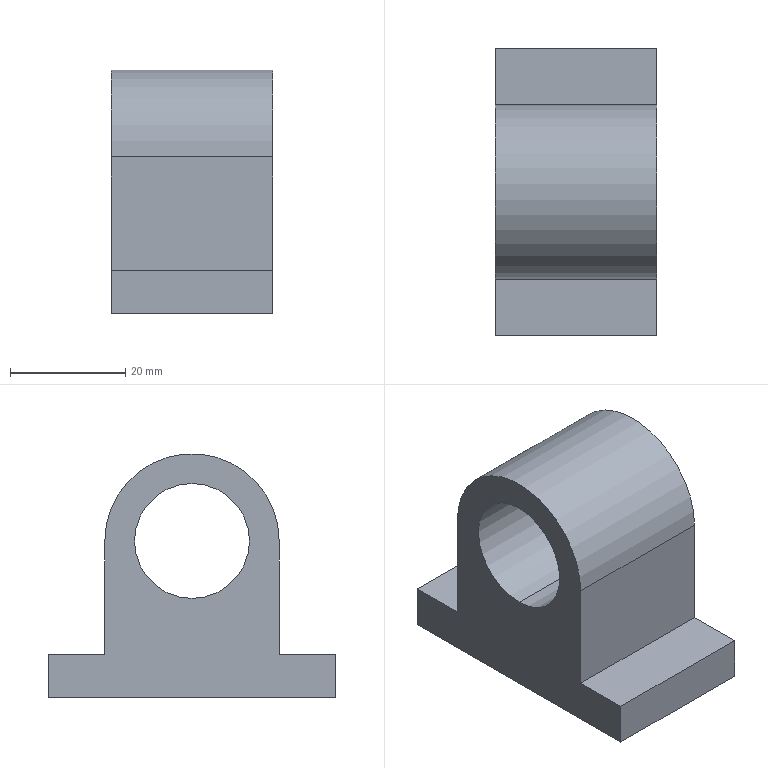Part | STEP file | 1 solid | 12 faces | box 28 x 50 x 42.426 mm | volume 28637 mm3 | plane 9 | cylinder 3 | commonest cylinder face diameters 20 x2 30.309 x1
STEP:
#1=CARTESIAN_POINT('',(0.,0.,0.));
#2=DIRECTION('',(0.,0.,1.));
#3=DIRECTION('',(1.,0.,0.));
#4=AXIS2_PLACEMENT_3D('',#1,#2,#3);
#5=CARTESIAN_POINT('',(572.,553.5,94.906));
#6=VERTEX_POINT('',#5);
#7=CARTESIAN_POINT('',(600.,553.5,94.906));
#8=VERTEX_POINT('',#7);
#9=CARTESIAN_POINT('',(572.,553.5,94.906));
#10=DIRECTION('',(1.,0.,0.));
#11=VECTOR('',#10,1.);
#12=LINE('',#9,#11);
#13=CARTESIAN_POINT('',(572.,553.5,104.906));
#14=DIRECTION('',(1.,0.,0.));
#15=DIRECTION('',(0.,0.,-1.));
#16=AXIS2_PLACEMENT_3D('',#13,#14,#15);
#17=CYLINDRICAL_SURFACE('',#16,10.);
#18=CARTESIAN_POINT('',(6.283,0.));
#19=DIRECTION('',(0.,1.));
#20=VECTOR('',#19,1.);
#21=LINE('',#18,#20);
#22=(GEOMETRIC_REPRESENTATION_CONTEXT(2)PARAMETRIC_REPRESENTATION_CONTEXT()REPRESENTATION_CONTEXT('',''));
#23=DEFINITIONAL_REPRESENTATION('',(#21),#22);
#24=PCURVE('',#17,#23);
#25=CARTESIAN_POINT('',(572.,553.5,104.906));
#26=DIRECTION('',(1.,0.,0.));
#27=DIRECTION('',(0.,0.,-1.));
#28=AXIS2_PLACEMENT_3D('',#25,#26,#27);
#29=CYLINDRICAL_SURFACE('',#28,10.);
#30=CARTESIAN_POINT('',(0.,0.));
#31=DIRECTION('',(0.,1.));
#32=VECTOR('',#31,1.);
#33=LINE('',#30,#32);
#34=(GEOMETRIC_REPRESENTATION_CONTEXT(2)PARAMETRIC_REPRESENTATION_CONTEXT()REPRESENTATION_CONTEXT('',''));
#35=DEFINITIONAL_REPRESENTATION('',(#33),#34);
#36=PCURVE('',#29,#35);
#37=SURFACE_CURVE('',#12,(#24,#36),.PCURVE_S1.);
#38=EDGE_CURVE('',#6,#8,#37,.T.);
#39=ORIENTED_EDGE('',*,*,#38,.T.);
#40=CARTESIAN_POINT('',(600.,553.5,114.906));
#41=VERTEX_POINT('',#40);
#42=CARTESIAN_POINT('',(600.,553.5,104.906));
#43=DIRECTION('',(1.,0.,0.));
#44=DIRECTION('',(0.,0.,-1.));
#45=AXIS2_PLACEMENT_3D('',#42,#43,#44);
#46=CIRCLE('',#45,10.);
#47=CARTESIAN_POINT('',(0.,28.));
#48=DIRECTION('',(1.,0.));
#49=VECTOR('',#48,1.);
#50=LINE('',#47,#49);
#51=(GEOMETRIC_REPRESENTATION_CONTEXT(2)PARAMETRIC_REPRESENTATION_CONTEXT()REPRESENTATION_CONTEXT('',''));
#52=DEFINITIONAL_REPRESENTATION('',(#50),#51);
#53=PCURVE('',#17,#52);
#54=CARTESIAN_POINT('',(600.,553.5,104.906));
#55=DIRECTION('',(1.,0.,0.));
#56=DIRECTION('',(0.,0.,-1.));
#57=AXIS2_PLACEMENT_3D('',#54,#55,#56);
#58=PLANE('',#57);
#59=CARTESIAN_POINT('',(0.,0.));
#60=DIRECTION('',(1.,0.));
#61=AXIS2_PLACEMENT_2D('',#59,#60);
#62=CIRCLE('',#61,10.);
#63=(GEOMETRIC_REPRESENTATION_CONTEXT(2)PARAMETRIC_REPRESENTATION_CONTEXT()REPRESENTATION_CONTEXT('',''));
#64=DEFINITIONAL_REPRESENTATION('',(#62),#63);
#65=PCURVE('',#58,#64);
#66=SURFACE_CURVE('',#46,(#53,#65),.PCURVE_S1.);
#67=EDGE_CURVE('',#41,#8,#66,.T.);
#68=ORIENTED_EDGE('',*,*,#67,.F.);
#69=CARTESIAN_POINT('',(572.,553.5,114.906));
#70=VERTEX_POINT('',#69);
#71=CARTESIAN_POINT('',(572.,553.5,114.906));
#72=DIRECTION('',(1.,0.,0.));
#73=VECTOR('',#72,1.);
#74=LINE('',#71,#73);
#75=CARTESIAN_POINT('',(3.142,0.));
#76=DIRECTION('',(0.,1.));
#77=VECTOR('',#76,1.);
#78=LINE('',#75,#77);
#79=(GEOMETRIC_REPRESENTATION_CONTEXT(2)PARAMETRIC_REPRESENTATION_CONTEXT()REPRESENTATION_CONTEXT('',''));
#80=DEFINITIONAL_REPRESENTATION('',(#78),#79);
#81=PCURVE('',#17,#80);
#82=CARTESIAN_POINT('',(3.142,0.));
#83=DIRECTION('',(0.,1.));
#84=VECTOR('',#83,1.);
#85=LINE('',#82,#84);
#86=(GEOMETRIC_REPRESENTATION_CONTEXT(2)PARAMETRIC_REPRESENTATION_CONTEXT()REPRESENTATION_CONTEXT('',''));
#87=DEFINITIONAL_REPRESENTATION('',(#85),#86);
#88=PCURVE('',#29,#87);
#89=SURFACE_CURVE('',#74,(#81,#88),.PCURVE_S1.);
#90=EDGE_CURVE('',#70,#41,#89,.T.);
#91=ORIENTED_EDGE('',*,*,#90,.F.);
#92=CARTESIAN_POINT('',(572.,553.5,104.906));
#93=DIRECTION('',(1.,0.,0.));
#94=DIRECTION('',(0.,0.,-1.));
#95=AXIS2_PLACEMENT_3D('',#92,#93,#94);
#96=CIRCLE('',#95,10.);
#97=CARTESIAN_POINT('',(0.,0.));
#98=DIRECTION('',(1.,0.));
#99=VECTOR('',#98,1.);
#100=LINE('',#97,#99);
#101=(GEOMETRIC_REPRESENTATION_CONTEXT(2)PARAMETRIC_REPRESENTATION_CONTEXT()REPRESENTATION_CONTEXT('',''));
#102=DEFINITIONAL_REPRESENTATION('',(#100),#101);
#103=PCURVE('',#17,#102);
#104=CARTESIAN_POINT('',(572.,553.5,104.906));
#105=DIRECTION('',(1.,0.,0.));
#106=DIRECTION('',(0.,0.,-1.));
#107=AXIS2_PLACEMENT_3D('',#104,#105,#106);
#108=PLANE('',#107);
#109=CARTESIAN_POINT('',(0.,0.));
#110=DIRECTION('',(1.,0.));
#111=AXIS2_PLACEMENT_2D('',#109,#110);
#112=CIRCLE('',#111,10.);
#113=(GEOMETRIC_REPRESENTATION_CONTEXT(2)PARAMETRIC_REPRESENTATION_CONTEXT()REPRESENTATION_CONTEXT('',''));
#114=DEFINITIONAL_REPRESENTATION('',(#112),#113);
#115=PCURVE('',#108,#114);
#116=SURFACE_CURVE('',#96,(#103,#115),.PCURVE_S1.);
#117=EDGE_CURVE('',#70,#6,#116,.T.);
#118=ORIENTED_EDGE('',*,*,#117,.T.);
#119=EDGE_LOOP('',(#39,#68,#91,#118));
#120=FACE_BOUND('',#119,.F.);
#121=ADVANCED_FACE('',(#120),#17,.F.);
#122=CARTESIAN_POINT('',(600.,528.5,77.635));
#123=VERTEX_POINT('',#122);
#124=CARTESIAN_POINT('',(600.,578.5,77.635));
#125=VERTEX_POINT('',#124);
#126=CARTESIAN_POINT('',(600.,578.5,77.635));
#127=DIRECTION('',(0.,1.,0.));
#128=VECTOR('',#127,1.);
#129=LINE('',#126,#128);
#130=CARTESIAN_POINT('',(572.,578.5,77.635));
#131=DIRECTION('',(0.,0.,-1.));
#132=DIRECTION('',(-1.,0.,0.));
#133=AXIS2_PLACEMENT_3D('',#130,#131,#132);
#134=PLANE('',#133);
#135=CARTESIAN_POINT('',(-28.,0.));
#136=DIRECTION('',(0.,1.));
#137=VECTOR('',#136,1.);
#138=LINE('',#135,#137);
#139=(GEOMETRIC_REPRESENTATION_CONTEXT(2)PARAMETRIC_REPRESENTATION_CONTEXT()REPRESENTATION_CONTEXT('',''));
#140=DEFINITIONAL_REPRESENTATION('',(#138),#139);
#141=PCURVE('',#134,#140);
#142=CARTESIAN_POINT('',(27.271,25.));
#143=DIRECTION('',(0.,1.));
#144=VECTOR('',#143,1.);
#145=LINE('',#142,#144);
#146=(GEOMETRIC_REPRESENTATION_CONTEXT(2)PARAMETRIC_REPRESENTATION_CONTEXT()REPRESENTATION_CONTEXT('',''));
#147=DEFINITIONAL_REPRESENTATION('',(#145),#146);
#148=PCURVE('',#58,#147);
#149=SURFACE_CURVE('',#129,(#141,#148),.PCURVE_S1.);
#150=EDGE_CURVE('',#123,#125,#149,.T.);
#151=ORIENTED_EDGE('',*,*,#150,.F.);
#152=CARTESIAN_POINT('',(572.,528.5,77.635));
#153=VERTEX_POINT('',#152);
#154=CARTESIAN_POINT('',(572.,528.5,77.635));
#155=DIRECTION('',(1.,0.,0.));
#156=VECTOR('',#155,1.);
#157=LINE('',#154,#156);
#158=CARTESIAN_POINT('',(0.,-50.));
#159=DIRECTION('',(-1.,0.));
#160=VECTOR('',#159,1.);
#161=LINE('',#158,#160);
#162=(GEOMETRIC_REPRESENTATION_CONTEXT(2)PARAMETRIC_REPRESENTATION_CONTEXT()REPRESENTATION_CONTEXT('',''));
#163=DEFINITIONAL_REPRESENTATION('',(#161),#162);
#164=PCURVE('',#134,#163);
#165=CARTESIAN_POINT('',(572.,528.5,77.635));
#166=DIRECTION('',(0.,-1.,0.));
#167=DIRECTION('',(0.,0.,-1.));
#168=AXIS2_PLACEMENT_3D('',#165,#166,#167);
#169=PLANE('',#168);
#170=CARTESIAN_POINT('',(0.,0.));
#171=DIRECTION('',(0.,1.));
#172=VECTOR('',#171,1.);
#173=LINE('',#170,#172);
#174=(GEOMETRIC_REPRESENTATION_CONTEXT(2)PARAMETRIC_REPRESENTATION_CONTEXT()REPRESENTATION_CONTEXT('',''));
#175=DEFINITIONAL_REPRESENTATION('',(#173),#174);
#176=PCURVE('',#169,#175);
#177=SURFACE_CURVE('',#157,(#164,#176),.PCURVE_S1.);
#178=EDGE_CURVE('',#153,#123,#177,.T.);
#179=ORIENTED_EDGE('',*,*,#178,.F.);
#180=CARTESIAN_POINT('',(572.,578.5,77.635));
#181=VERTEX_POINT('',#180);
#182=CARTESIAN_POINT('',(572.,578.5,77.635));
#183=DIRECTION('',(0.,1.,0.));
#184=VECTOR('',#183,1.);
#185=LINE('',#182,#184);
#186=CARTESIAN_POINT('',(0.,0.));
#187=DIRECTION('',(0.,1.));
#188=VECTOR('',#187,1.);
#189=LINE('',#186,#188);
#190=(GEOMETRIC_REPRESENTATION_CONTEXT(2)PARAMETRIC_REPRESENTATION_CONTEXT()REPRESENTATION_CONTEXT('',''));
#191=DEFINITIONAL_REPRESENTATION('',(#189),#190);
#192=PCURVE('',#134,#191);
#193=CARTESIAN_POINT('',(27.271,25.));
#194=DIRECTION('',(0.,1.));
#195=VECTOR('',#194,1.);
#196=LINE('',#193,#195);
#197=(GEOMETRIC_REPRESENTATION_CONTEXT(2)PARAMETRIC_REPRESENTATION_CONTEXT()REPRESENTATION_CONTEXT('',''));
#198=DEFINITIONAL_REPRESENTATION('',(#196),#197);
#199=PCURVE('',#108,#198);
#200=SURFACE_CURVE('',#185,(#192,#199),.PCURVE_S1.);
#201=EDGE_CURVE('',#153,#181,#200,.T.);
#202=ORIENTED_EDGE('',*,*,#201,.T.);
#203=CARTESIAN_POINT('',(572.,578.5,77.635));
#204=DIRECTION('',(1.,0.,0.));
#205=VECTOR('',#204,1.);
#206=LINE('',#203,#205);
#207=CARTESIAN_POINT('',(0.,0.));
#208=DIRECTION('',(-1.,0.));
#209=VECTOR('',#208,1.);
#210=LINE('',#207,#209);
#211=(GEOMETRIC_REPRESENTATION_CONTEXT(2)PARAMETRIC_REPRESENTATION_CONTEXT()REPRESENTATION_CONTEXT('',''));
#212=DEFINITIONAL_REPRESENTATION('',(#210),#211);
#213=PCURVE('',#134,#212);
#214=CARTESIAN_POINT('',(572.,578.5,77.635));
#215=DIRECTION('',(0.,1.,0.));
#216=DIRECTION('',(0.,0.,1.));
#217=AXIS2_PLACEMENT_3D('',#214,#215,#216);
#218=PLANE('',#217);
#219=CARTESIAN_POINT('',(0.,0.));
#220=DIRECTION('',(0.,1.));
#221=VECTOR('',#220,1.);
#222=LINE('',#219,#221);
#223=(GEOMETRIC_REPRESENTATION_CONTEXT(2)PARAMETRIC_REPRESENTATION_CONTEXT()REPRESENTATION_CONTEXT('',''));
#224=DEFINITIONAL_REPRESENTATION('',(#222),#223);
#225=PCURVE('',#218,#224);
#226=SURFACE_CURVE('',#206,(#213,#225),.PCURVE_S1.);
#227=EDGE_CURVE('',#181,#125,#226,.T.);
#228=ORIENTED_EDGE('',*,*,#227,.T.);
#229=EDGE_LOOP('',(#151,#179,#202,#228));
#230=FACE_BOUND('',#229,.T.);
#231=ADVANCED_FACE('',(#230),#134,.T.);
#232=CARTESIAN_POINT('',(600.,528.5,85.232));
#233=VERTEX_POINT('',#232);
#234=CARTESIAN_POINT('',(600.,528.5,77.635));
#235=DIRECTION('',(0.,0.,-1.));
#236=VECTOR('',#235,1.);
#237=LINE('',#234,#236);
#238=CARTESIAN_POINT('',(0.,28.));
#239=DIRECTION('',(1.,0.));
#240=VECTOR('',#239,1.);
#241=LINE('',#238,#240);
#242=(GEOMETRIC_REPRESENTATION_CONTEXT(2)PARAMETRIC_REPRESENTATION_CONTEXT()REPRESENTATION_CONTEXT('',''));
#243=DEFINITIONAL_REPRESENTATION('',(#241),#242);
#244=PCURVE('',#169,#243);
#245=CARTESIAN_POINT('',(27.271,-25.));
#246=DIRECTION('',(1.,0.));
#247=VECTOR('',#246,1.);
#248=LINE('',#245,#247);
#249=(GEOMETRIC_REPRESENTATION_CONTEXT(2)PARAMETRIC_REPRESENTATION_CONTEXT()REPRESENTATION_CONTEXT('',''));
#250=DEFINITIONAL_REPRESENTATION('',(#248),#249);
#251=PCURVE('',#58,#250);
#252=SURFACE_CURVE('',#237,(#244,#251),.PCURVE_S1.);
#253=EDGE_CURVE('',#233,#123,#252,.T.);
#254=ORIENTED_EDGE('',*,*,#253,.F.);
#255=CARTESIAN_POINT('',(572.,528.5,85.232));
#256=VERTEX_POINT('',#255);
#257=CARTESIAN_POINT('',(572.,528.5,85.232));
#258=DIRECTION('',(1.,0.,0.));
#259=VECTOR('',#258,1.);
#260=LINE('',#257,#259);
#261=CARTESIAN_POINT('',(-7.597,0.));
#262=DIRECTION('',(0.,1.));
#263=VECTOR('',#262,1.);
#264=LINE('',#261,#263);
#265=(GEOMETRIC_REPRESENTATION_CONTEXT(2)PARAMETRIC_REPRESENTATION_CONTEXT()REPRESENTATION_CONTEXT('',''));
#266=DEFINITIONAL_REPRESENTATION('',(#264),#265);
#267=PCURVE('',#169,#266);
#268=CARTESIAN_POINT('',(572.,538.345,85.232));
#269=DIRECTION('',(0.,0.,1.));
#270=DIRECTION('',(1.,0.,0.));
#271=AXIS2_PLACEMENT_3D('',#268,#269,#270);
#272=PLANE('',#271);
#273=CARTESIAN_POINT('',(0.,-9.845));
#274=DIRECTION('',(1.,0.));
#275=VECTOR('',#274,1.);
#276=LINE('',#273,#275);
#277=(GEOMETRIC_REPRESENTATION_CONTEXT(2)PARAMETRIC_REPRESENTATION_CONTEXT()REPRESENTATION_CONTEXT('',''));
#278=DEFINITIONAL_REPRESENTATION('',(#276),#277);
#279=PCURVE('',#272,#278);
#280=SURFACE_CURVE('',#260,(#267,#279),.PCURVE_S1.);
#281=EDGE_CURVE('',#256,#233,#280,.T.);
#282=ORIENTED_EDGE('',*,*,#281,.F.);
#283=CARTESIAN_POINT('',(572.,528.5,77.635));
#284=DIRECTION('',(0.,0.,-1.));
#285=VECTOR('',#284,1.);
#286=LINE('',#283,#285);
#287=CARTESIAN_POINT('',(0.,0.));
#288=DIRECTION('',(1.,0.));
#289=VECTOR('',#288,1.);
#290=LINE('',#287,#289);
#291=(GEOMETRIC_REPRESENTATION_CONTEXT(2)PARAMETRIC_REPRESENTATION_CONTEXT()REPRESENTATION_CONTEXT('',''));
#292=DEFINITIONAL_REPRESENTATION('',(#290),#291);
#293=PCURVE('',#169,#292);
#294=CARTESIAN_POINT('',(27.271,-25.));
#295=DIRECTION('',(1.,0.));
#296=VECTOR('',#295,1.);
#297=LINE('',#294,#296);
#298=(GEOMETRIC_REPRESENTATION_CONTEXT(2)PARAMETRIC_REPRESENTATION_CONTEXT()REPRESENTATION_CONTEXT('',''));
#299=DEFINITIONAL_REPRESENTATION('',(#297),#298);
#300=PCURVE('',#108,#299);
#301=SURFACE_CURVE('',#286,(#293,#300),.PCURVE_S1.);
#302=EDGE_CURVE('',#256,#153,#301,.T.);
#303=ORIENTED_EDGE('',*,*,#302,.T.);
#304=ORIENTED_EDGE('',*,*,#178,.T.);
#305=EDGE_LOOP('',(#254,#282,#303,#304));
#306=FACE_BOUND('',#305,.T.);
#307=ADVANCED_FACE('',(#306),#169,.T.);
#308=CARTESIAN_POINT('',(600.,538.345,85.232));
#309=VERTEX_POINT('',#308);
#310=CARTESIAN_POINT('',(600.,538.345,85.232));
#311=DIRECTION('',(0.,-1.,0.));
#312=VECTOR('',#311,1.);
#313=LINE('',#310,#312);
#314=CARTESIAN_POINT('',(28.,0.));
#315=DIRECTION('',(0.,-1.));
#316=VECTOR('',#315,1.);
#317=LINE('',#314,#316);
#318=(GEOMETRIC_REPRESENTATION_CONTEXT(2)PARAMETRIC_REPRESENTATION_CONTEXT()REPRESENTATION_CONTEXT('',''));
#319=DEFINITIONAL_REPRESENTATION('',(#317),#318);
#320=PCURVE('',#272,#319);
#321=CARTESIAN_POINT('',(19.674,-15.155));
#322=DIRECTION('',(0.,-1.));
#323=VECTOR('',#322,1.);
#324=LINE('',#321,#323);
#325=(GEOMETRIC_REPRESENTATION_CONTEXT(2)PARAMETRIC_REPRESENTATION_CONTEXT()REPRESENTATION_CONTEXT('',''));
#326=DEFINITIONAL_REPRESENTATION('',(#324),#325);
#327=PCURVE('',#58,#326);
#328=SURFACE_CURVE('',#313,(#320,#327),.PCURVE_S1.);
#329=EDGE_CURVE('',#309,#233,#328,.T.);
#330=ORIENTED_EDGE('',*,*,#329,.F.);
#331=CARTESIAN_POINT('',(572.,538.345,85.232));
#332=VERTEX_POINT('',#331);
#333=CARTESIAN_POINT('',(572.,538.345,85.232));
#334=DIRECTION('',(1.,0.,0.));
#335=VECTOR('',#334,1.);
#336=LINE('',#333,#335);
#337=CARTESIAN_POINT('',(0.,0.));
#338=DIRECTION('',(1.,0.));
#339=VECTOR('',#338,1.);
#340=LINE('',#337,#339);
#341=(GEOMETRIC_REPRESENTATION_CONTEXT(2)PARAMETRIC_REPRESENTATION_CONTEXT()REPRESENTATION_CONTEXT('',''));
#342=DEFINITIONAL_REPRESENTATION('',(#340),#341);
#343=PCURVE('',#272,#342);
#344=CARTESIAN_POINT('',(572.,538.345,104.906));
#345=DIRECTION('',(0.,-1.,0.));
#346=DIRECTION('',(0.,0.,-1.));
#347=AXIS2_PLACEMENT_3D('',#344,#345,#346);
#348=PLANE('',#347);
#349=CARTESIAN_POINT('',(19.674,0.));
#350=DIRECTION('',(0.,1.));
#351=VECTOR('',#350,1.);
#352=LINE('',#349,#351);
#353=(GEOMETRIC_REPRESENTATION_CONTEXT(2)PARAMETRIC_REPRESENTATION_CONTEXT()REPRESENTATION_CONTEXT('',''));
#354=DEFINITIONAL_REPRESENTATION('',(#352),#353);
#355=PCURVE('',#348,#354);
#356=SURFACE_CURVE('',#336,(#343,#355),.PCURVE_S1.);
#357=EDGE_CURVE('',#332,#309,#356,.T.);
#358=ORIENTED_EDGE('',*,*,#357,.F.);
#359=CARTESIAN_POINT('',(572.,538.345,85.232));
#360=DIRECTION('',(0.,-1.,0.));
#361=VECTOR('',#360,1.);
#362=LINE('',#359,#361);
#363=CARTESIAN_POINT('',(0.,0.));
#364=DIRECTION('',(0.,-1.));
#365=VECTOR('',#364,1.);
#366=LINE('',#363,#365);
#367=(GEOMETRIC_REPRESENTATION_CONTEXT(2)PARAMETRIC_REPRESENTATION_CONTEXT()REPRESENTATION_CONTEXT('',''));
#368=DEFINITIONAL_REPRESENTATION('',(#366),#367);
#369=PCURVE('',#272,#368);
#370=CARTESIAN_POINT('',(19.674,-15.155));
#371=DIRECTION('',(0.,-1.));
#372=VECTOR('',#371,1.);
#373=LINE('',#370,#372);
#374=(GEOMETRIC_REPRESENTATION_CONTEXT(2)PARAMETRIC_REPRESENTATION_CONTEXT()REPRESENTATION_CONTEXT('',''));
#375=DEFINITIONAL_REPRESENTATION('',(#373),#374);
#376=PCURVE('',#108,#375);
#377=SURFACE_CURVE('',#362,(#369,#376),.PCURVE_S1.);
#378=EDGE_CURVE('',#332,#256,#377,.T.);
#379=ORIENTED_EDGE('',*,*,#378,.T.);
#380=ORIENTED_EDGE('',*,*,#281,.T.);
#381=EDGE_LOOP('',(#330,#358,#379,#380));
#382=FACE_BOUND('',#381,.T.);
#383=ADVANCED_FACE('',(#382),#272,.T.);
#384=CARTESIAN_POINT('',(600.,538.345,104.906));
#385=VERTEX_POINT('',#384);
#386=CARTESIAN_POINT('',(600.,538.345,104.906));
#387=DIRECTION('',(0.,0.,-1.));
#388=VECTOR('',#387,1.);
#389=LINE('',#386,#388);
#390=CARTESIAN_POINT('',(0.,28.));
#391=DIRECTION('',(1.,0.));
#392=VECTOR('',#391,1.);
#393=LINE('',#390,#392);
#394=(GEOMETRIC_REPRESENTATION_CONTEXT(2)PARAMETRIC_REPRESENTATION_CONTEXT()REPRESENTATION_CONTEXT('',''));
#395=DEFINITIONAL_REPRESENTATION('',(#393),#394);
#396=PCURVE('',#348,#395);
#397=CARTESIAN_POINT('',(0.,-15.155));
#398=DIRECTION('',(1.,0.));
#399=VECTOR('',#398,1.);
#400=LINE('',#397,#399);
#401=(GEOMETRIC_REPRESENTATION_CONTEXT(2)PARAMETRIC_REPRESENTATION_CONTEXT()REPRESENTATION_CONTEXT('',''));
#402=DEFINITIONAL_REPRESENTATION('',(#400),#401);
#403=PCURVE('',#58,#402);
#404=SURFACE_CURVE('',#389,(#396,#403),.PCURVE_S1.);
#405=EDGE_CURVE('',#385,#309,#404,.T.);
#406=ORIENTED_EDGE('',*,*,#405,.F.);
#407=CARTESIAN_POINT('',(572.,538.345,104.906));
#408=VERTEX_POINT('',#407);
#409=CARTESIAN_POINT('',(572.,538.345,104.906));
#410=DIRECTION('',(1.,0.,0.));
#411=VECTOR('',#410,1.);
#412=LINE('',#409,#411);
#413=CARTESIAN_POINT('',(0.,0.));
#414=DIRECTION('',(0.,1.));
#415=VECTOR('',#414,1.);
#416=LINE('',#413,#415);
#417=(GEOMETRIC_REPRESENTATION_CONTEXT(2)PARAMETRIC_REPRESENTATION_CONTEXT()REPRESENTATION_CONTEXT('',''));
#418=DEFINITIONAL_REPRESENTATION('',(#416),#417);
#419=PCURVE('',#348,#418);
#420=CARTESIAN_POINT('',(572.,553.5,104.906));
#421=DIRECTION('',(1.,0.,0.));
#422=DIRECTION('',(0.,0.,-1.));
#423=AXIS2_PLACEMENT_3D('',#420,#421,#422);
#424=CYLINDRICAL_SURFACE('',#423,15.155);
#425=CARTESIAN_POINT('',(4.712,0.));
#426=DIRECTION('',(0.,1.));
#427=VECTOR('',#426,1.);
#428=LINE('',#425,#427);
#429=(GEOMETRIC_REPRESENTATION_CONTEXT(2)PARAMETRIC_REPRESENTATION_CONTEXT()REPRESENTATION_CONTEXT('',''));
#430=DEFINITIONAL_REPRESENTATION('',(#428),#429);
#431=PCURVE('',#424,#430);
#432=SURFACE_CURVE('',#412,(#419,#431),.PCURVE_S1.);
#433=EDGE_CURVE('',#408,#385,#432,.T.);
#434=ORIENTED_EDGE('',*,*,#433,.F.);
#435=CARTESIAN_POINT('',(572.,538.345,104.906));
#436=DIRECTION('',(0.,0.,-1.));
#437=VECTOR('',#436,1.);
#438=LINE('',#435,#437);
#439=CARTESIAN_POINT('',(0.,0.));
#440=DIRECTION('',(1.,0.));
#441=VECTOR('',#440,1.);
#442=LINE('',#439,#441);
#443=(GEOMETRIC_REPRESENTATION_CONTEXT(2)PARAMETRIC_REPRESENTATION_CONTEXT()REPRESENTATION_CONTEXT('',''));
#444=DEFINITIONAL_REPRESENTATION('',(#442),#443);
#445=PCURVE('',#348,#444);
#446=CARTESIAN_POINT('',(0.,-15.155));
#447=DIRECTION('',(1.,0.));
#448=VECTOR('',#447,1.);
#449=LINE('',#446,#448);
#450=(GEOMETRIC_REPRESENTATION_CONTEXT(2)PARAMETRIC_REPRESENTATION_CONTEXT()REPRESENTATION_CONTEXT('',''));
#451=DEFINITIONAL_REPRESENTATION('',(#449),#450);
#452=PCURVE('',#108,#451);
#453=SURFACE_CURVE('',#438,(#445,#452),.PCURVE_S1.);
#454=EDGE_CURVE('',#408,#332,#453,.T.);
#455=ORIENTED_EDGE('',*,*,#454,.T.);
#456=ORIENTED_EDGE('',*,*,#357,.T.);
#457=EDGE_LOOP('',(#406,#434,#455,#456));
#458=FACE_BOUND('',#457,.T.);
#459=ADVANCED_FACE('',(#458),#348,.T.);
#460=CARTESIAN_POINT('',(600.,568.655,104.906));
#461=VERTEX_POINT('',#460);
#462=CARTESIAN_POINT('',(600.,553.5,104.906));
#463=DIRECTION('',(1.,0.,0.));
#464=DIRECTION('',(0.,0.,-1.));
#465=AXIS2_PLACEMENT_3D('',#462,#463,#464);
#466=CIRCLE('',#465,15.155);
#467=CARTESIAN_POINT('',(0.,28.));
#468=DIRECTION('',(1.,0.));
#469=VECTOR('',#468,1.);
#470=LINE('',#467,#469);
#471=(GEOMETRIC_REPRESENTATION_CONTEXT(2)PARAMETRIC_REPRESENTATION_CONTEXT()REPRESENTATION_CONTEXT('',''));
#472=DEFINITIONAL_REPRESENTATION('',(#470),#471);
#473=PCURVE('',#424,#472);
#474=CARTESIAN_POINT('',(0.,0.));
#475=DIRECTION('',(1.,0.));
#476=AXIS2_PLACEMENT_2D('',#474,#475);
#477=CIRCLE('',#476,15.155);
#478=(GEOMETRIC_REPRESENTATION_CONTEXT(2)PARAMETRIC_REPRESENTATION_CONTEXT()REPRESENTATION_CONTEXT('',''));
#479=DEFINITIONAL_REPRESENTATION('',(#477),#478);
#480=PCURVE('',#58,#479);
#481=SURFACE_CURVE('',#466,(#473,#480),.PCURVE_S1.);
#482=EDGE_CURVE('',#461,#385,#481,.T.);
#483=ORIENTED_EDGE('',*,*,#482,.F.);
#484=CARTESIAN_POINT('',(572.,568.655,104.906));
#485=VERTEX_POINT('',#484);
#486=CARTESIAN_POINT('',(572.,568.655,104.906));
#487=DIRECTION('',(1.,0.,0.));
#488=VECTOR('',#487,1.);
#489=LINE('',#486,#488);
#490=CARTESIAN_POINT('',(1.571,0.));
#491=DIRECTION('',(0.,1.));
#492=VECTOR('',#491,1.);
#493=LINE('',#490,#492);
#494=(GEOMETRIC_REPRESENTATION_CONTEXT(2)PARAMETRIC_REPRESENTATION_CONTEXT()REPRESENTATION_CONTEXT('',''));
#495=DEFINITIONAL_REPRESENTATION('',(#493),#494);
#496=PCURVE('',#424,#495);
#497=CARTESIAN_POINT('',(572.,568.655,104.906));
#498=DIRECTION('',(0.,1.,0.));
#499=DIRECTION('',(0.,0.,1.));
#500=AXIS2_PLACEMENT_3D('',#497,#498,#499);
#501=PLANE('',#500);
#502=CARTESIAN_POINT('',(0.,0.));
#503=DIRECTION('',(0.,1.));
#504=VECTOR('',#503,1.);
#505=LINE('',#502,#504);
#506=(GEOMETRIC_REPRESENTATION_CONTEXT(2)PARAMETRIC_REPRESENTATION_CONTEXT()REPRESENTATION_CONTEXT('',''));
#507=DEFINITIONAL_REPRESENTATION('',(#505),#506);
#508=PCURVE('',#501,#507);
#509=SURFACE_CURVE('',#489,(#496,#508),.PCURVE_S1.);
#510=EDGE_CURVE('',#485,#461,#509,.T.);
#511=ORIENTED_EDGE('',*,*,#510,.F.);
#512=CARTESIAN_POINT('',(572.,553.5,104.906));
#513=DIRECTION('',(1.,0.,0.));
#514=DIRECTION('',(0.,0.,-1.));
#515=AXIS2_PLACEMENT_3D('',#512,#513,#514);
#516=CIRCLE('',#515,15.155);
#517=CARTESIAN_POINT('',(0.,0.));
#518=DIRECTION('',(1.,0.));
#519=VECTOR('',#518,1.);
#520=LINE('',#517,#519);
#521=(GEOMETRIC_REPRESENTATION_CONTEXT(2)PARAMETRIC_REPRESENTATION_CONTEXT()REPRESENTATION_CONTEXT('',''));
#522=DEFINITIONAL_REPRESENTATION('',(#520),#521);
#523=PCURVE('',#424,#522);
#524=CARTESIAN_POINT('',(0.,0.));
#525=DIRECTION('',(1.,0.));
#526=AXIS2_PLACEMENT_2D('',#524,#525);
#527=CIRCLE('',#526,15.155);
#528=(GEOMETRIC_REPRESENTATION_CONTEXT(2)PARAMETRIC_REPRESENTATION_CONTEXT()REPRESENTATION_CONTEXT('',''));
#529=DEFINITIONAL_REPRESENTATION('',(#527),#528);
#530=PCURVE('',#108,#529);
#531=SURFACE_CURVE('',#516,(#523,#530),.PCURVE_S1.);
#532=EDGE_CURVE('',#485,#408,#531,.T.);
#533=ORIENTED_EDGE('',*,*,#532,.T.);
#534=ORIENTED_EDGE('',*,*,#433,.T.);
#535=EDGE_LOOP('',(#483,#511,#533,#534));
#536=FACE_BOUND('',#535,.T.);
#537=ADVANCED_FACE('',(#536),#424,.T.);
#538=CARTESIAN_POINT('',(600.,568.655,85.232));
#539=VERTEX_POINT('',#538);
#540=CARTESIAN_POINT('',(600.,568.655,104.906));
#541=DIRECTION('',(0.,0.,1.));
#542=VECTOR('',#541,1.);
#543=LINE('',#540,#542);
#544=CARTESIAN_POINT('',(0.,28.));
#545=DIRECTION('',(1.,0.));
#546=VECTOR('',#545,1.);
#547=LINE('',#544,#546);
#548=(GEOMETRIC_REPRESENTATION_CONTEXT(2)PARAMETRIC_REPRESENTATION_CONTEXT()REPRESENTATION_CONTEXT('',''));
#549=DEFINITIONAL_REPRESENTATION('',(#547),#548);
#550=PCURVE('',#501,#549);
#551=CARTESIAN_POINT('',(0.,15.155));
#552=DIRECTION('',(-1.,0.));
#553=VECTOR('',#552,1.);
#554=LINE('',#551,#553);
#555=(GEOMETRIC_REPRESENTATION_CONTEXT(2)PARAMETRIC_REPRESENTATION_CONTEXT()REPRESENTATION_CONTEXT('',''));
#556=DEFINITIONAL_REPRESENTATION('',(#554),#555);
#557=PCURVE('',#58,#556);
#558=SURFACE_CURVE('',#543,(#550,#557),.PCURVE_S1.);
#559=EDGE_CURVE('',#539,#461,#558,.T.);
#560=ORIENTED_EDGE('',*,*,#559,.F.);
#561=CARTESIAN_POINT('',(572.,568.655,85.232));
#562=VERTEX_POINT('',#561);
#563=CARTESIAN_POINT('',(572.,568.655,85.232));
#564=DIRECTION('',(1.,0.,0.));
#565=VECTOR('',#564,1.);
#566=LINE('',#563,#565);
#567=CARTESIAN_POINT('',(-19.674,0.));
#568=DIRECTION('',(0.,1.));
#569=VECTOR('',#568,1.);
#570=LINE('',#567,#569);
#571=(GEOMETRIC_REPRESENTATION_CONTEXT(2)PARAMETRIC_REPRESENTATION_CONTEXT()REPRESENTATION_CONTEXT('',''));
#572=DEFINITIONAL_REPRESENTATION('',(#570),#571);
#573=PCURVE('',#501,#572);
#574=CARTESIAN_POINT('',(572.,578.5,85.232));
#575=DIRECTION('',(0.,0.,1.));
#576=DIRECTION('',(1.,0.,0.));
#577=AXIS2_PLACEMENT_3D('',#574,#575,#576);
#578=PLANE('',#577);
#579=CARTESIAN_POINT('',(0.,-9.845));
#580=DIRECTION('',(1.,0.));
#581=VECTOR('',#580,1.);
#582=LINE('',#579,#581);
#583=(GEOMETRIC_REPRESENTATION_CONTEXT(2)PARAMETRIC_REPRESENTATION_CONTEXT()REPRESENTATION_CONTEXT('',''));
#584=DEFINITIONAL_REPRESENTATION('',(#582),#583);
#585=PCURVE('',#578,#584);
#586=SURFACE_CURVE('',#566,(#573,#585),.PCURVE_S1.);
#587=EDGE_CURVE('',#562,#539,#586,.T.);
#588=ORIENTED_EDGE('',*,*,#587,.F.);
#589=CARTESIAN_POINT('',(572.,568.655,104.906));
#590=DIRECTION('',(0.,0.,1.));
#591=VECTOR('',#590,1.);
#592=LINE('',#589,#591);
#593=CARTESIAN_POINT('',(0.,0.));
#594=DIRECTION('',(1.,0.));
#595=VECTOR('',#594,1.);
#596=LINE('',#593,#595);
#597=(GEOMETRIC_REPRESENTATION_CONTEXT(2)PARAMETRIC_REPRESENTATION_CONTEXT()REPRESENTATION_CONTEXT('',''));
#598=DEFINITIONAL_REPRESENTATION('',(#596),#597);
#599=PCURVE('',#501,#598);
#600=CARTESIAN_POINT('',(0.,15.155));
#601=DIRECTION('',(-1.,0.));
#602=VECTOR('',#601,1.);
#603=LINE('',#600,#602);
#604=(GEOMETRIC_REPRESENTATION_CONTEXT(2)PARAMETRIC_REPRESENTATION_CONTEXT()REPRESENTATION_CONTEXT('',''));
#605=DEFINITIONAL_REPRESENTATION('',(#603),#604);
#606=PCURVE('',#108,#605);
#607=SURFACE_CURVE('',#592,(#599,#606),.PCURVE_S1.);
#608=EDGE_CURVE('',#562,#485,#607,.T.);
#609=ORIENTED_EDGE('',*,*,#608,.T.);
#610=ORIENTED_EDGE('',*,*,#510,.T.);
#611=EDGE_LOOP('',(#560,#588,#609,#610));
#612=FACE_BOUND('',#611,.T.);
#613=ADVANCED_FACE('',(#612),#501,.T.);
#614=CARTESIAN_POINT('',(600.,578.5,85.232));
#615=VERTEX_POINT('',#614);
#616=CARTESIAN_POINT('',(600.,578.5,85.232));
#617=DIRECTION('',(0.,-1.,0.));
#618=VECTOR('',#617,1.);
#619=LINE('',#616,#618);
#620=CARTESIAN_POINT('',(28.,0.));
#621=DIRECTION('',(0.,-1.));
#622=VECTOR('',#621,1.);
#623=LINE('',#620,#622);
#624=(GEOMETRIC_REPRESENTATION_CONTEXT(2)PARAMETRIC_REPRESENTATION_CONTEXT()REPRESENTATION_CONTEXT('',''));
#625=DEFINITIONAL_REPRESENTATION('',(#623),#624);
#626=PCURVE('',#578,#625);
#627=CARTESIAN_POINT('',(19.674,25.));
#628=DIRECTION('',(0.,-1.));
#629=VECTOR('',#628,1.);
#630=LINE('',#627,#629);
#631=(GEOMETRIC_REPRESENTATION_CONTEXT(2)PARAMETRIC_REPRESENTATION_CONTEXT()REPRESENTATION_CONTEXT('',''));
#632=DEFINITIONAL_REPRESENTATION('',(#630),#631);
#633=PCURVE('',#58,#632);
#634=SURFACE_CURVE('',#619,(#626,#633),.PCURVE_S1.);
#635=EDGE_CURVE('',#615,#539,#634,.T.);
#636=ORIENTED_EDGE('',*,*,#635,.F.);
#637=CARTESIAN_POINT('',(572.,578.5,85.232));
#638=VERTEX_POINT('',#637);
#639=CARTESIAN_POINT('',(572.,578.5,85.232));
#640=DIRECTION('',(1.,0.,0.));
#641=VECTOR('',#640,1.);
#642=LINE('',#639,#641);
#643=CARTESIAN_POINT('',(0.,0.));
#644=DIRECTION('',(1.,0.));
#645=VECTOR('',#644,1.);
#646=LINE('',#643,#645);
#647=(GEOMETRIC_REPRESENTATION_CONTEXT(2)PARAMETRIC_REPRESENTATION_CONTEXT()REPRESENTATION_CONTEXT('',''));
#648=DEFINITIONAL_REPRESENTATION('',(#646),#647);
#649=PCURVE('',#578,#648);
#650=CARTESIAN_POINT('',(7.597,0.));
#651=DIRECTION('',(0.,1.));
#652=VECTOR('',#651,1.);
#653=LINE('',#650,#652);
#654=(GEOMETRIC_REPRESENTATION_CONTEXT(2)PARAMETRIC_REPRESENTATION_CONTEXT()REPRESENTATION_CONTEXT('',''));
#655=DEFINITIONAL_REPRESENTATION('',(#653),#654);
#656=PCURVE('',#218,#655);
#657=SURFACE_CURVE('',#642,(#649,#656),.PCURVE_S1.);
#658=EDGE_CURVE('',#638,#615,#657,.T.);
#659=ORIENTED_EDGE('',*,*,#658,.F.);
#660=CARTESIAN_POINT('',(572.,578.5,85.232));
#661=DIRECTION('',(0.,-1.,0.));
#662=VECTOR('',#661,1.);
#663=LINE('',#660,#662);
#664=CARTESIAN_POINT('',(0.,0.));
#665=DIRECTION('',(0.,-1.));
#666=VECTOR('',#665,1.);
#667=LINE('',#664,#666);
#668=(GEOMETRIC_REPRESENTATION_CONTEXT(2)PARAMETRIC_REPRESENTATION_CONTEXT()REPRESENTATION_CONTEXT('',''));
#669=DEFINITIONAL_REPRESENTATION('',(#667),#668);
#670=PCURVE('',#578,#669);
#671=CARTESIAN_POINT('',(19.674,25.));
#672=DIRECTION('',(0.,-1.));
#673=VECTOR('',#672,1.);
#674=LINE('',#671,#673);
#675=(GEOMETRIC_REPRESENTATION_CONTEXT(2)PARAMETRIC_REPRESENTATION_CONTEXT()REPRESENTATION_CONTEXT('',''));
#676=DEFINITIONAL_REPRESENTATION('',(#674),#675);
#677=PCURVE('',#108,#676);
#678=SURFACE_CURVE('',#663,(#670,#677),.PCURVE_S1.);
#679=EDGE_CURVE('',#638,#562,#678,.T.);
#680=ORIENTED_EDGE('',*,*,#679,.T.);
#681=ORIENTED_EDGE('',*,*,#587,.T.);
#682=EDGE_LOOP('',(#636,#659,#680,#681));
#683=FACE_BOUND('',#682,.T.);
#684=ADVANCED_FACE('',(#683),#578,.T.);
#685=CARTESIAN_POINT('',(600.,578.5,77.635));
#686=DIRECTION('',(0.,0.,1.));
#687=VECTOR('',#686,1.);
#688=LINE('',#685,#687);
#689=CARTESIAN_POINT('',(0.,28.));
#690=DIRECTION('',(1.,0.));
#691=VECTOR('',#690,1.);
#692=LINE('',#689,#691);
#693=(GEOMETRIC_REPRESENTATION_CONTEXT(2)PARAMETRIC_REPRESENTATION_CONTEXT()REPRESENTATION_CONTEXT('',''));
#694=DEFINITIONAL_REPRESENTATION('',(#692),#693);
#695=PCURVE('',#218,#694);
#696=CARTESIAN_POINT('',(27.271,25.));
#697=DIRECTION('',(-1.,0.));
#698=VECTOR('',#697,1.);
#699=LINE('',#696,#698);
#700=(GEOMETRIC_REPRESENTATION_CONTEXT(2)PARAMETRIC_REPRESENTATION_CONTEXT()REPRESENTATION_CONTEXT('',''));
#701=DEFINITIONAL_REPRESENTATION('',(#699),#700);
#702=PCURVE('',#58,#701);
#703=SURFACE_CURVE('',#688,(#695,#702),.PCURVE_S1.);
#704=EDGE_CURVE('',#125,#615,#703,.T.);
#705=ORIENTED_EDGE('',*,*,#704,.F.);
#706=ORIENTED_EDGE('',*,*,#227,.F.);
#707=CARTESIAN_POINT('',(572.,578.5,77.635));
#708=DIRECTION('',(0.,0.,1.));
#709=VECTOR('',#708,1.);
#710=LINE('',#707,#709);
#711=CARTESIAN_POINT('',(0.,0.));
#712=DIRECTION('',(1.,0.));
#713=VECTOR('',#712,1.);
#714=LINE('',#711,#713);
#715=(GEOMETRIC_REPRESENTATION_CONTEXT(2)PARAMETRIC_REPRESENTATION_CONTEXT()REPRESENTATION_CONTEXT('',''));
#716=DEFINITIONAL_REPRESENTATION('',(#714),#715);
#717=PCURVE('',#218,#716);
#718=CARTESIAN_POINT('',(27.271,25.));
#719=DIRECTION('',(-1.,0.));
#720=VECTOR('',#719,1.);
#721=LINE('',#718,#720);
#722=(GEOMETRIC_REPRESENTATION_CONTEXT(2)PARAMETRIC_REPRESENTATION_CONTEXT()REPRESENTATION_CONTEXT('',''));
#723=DEFINITIONAL_REPRESENTATION('',(#721),#722);
#724=PCURVE('',#108,#723);
#725=SURFACE_CURVE('',#710,(#717,#724),.PCURVE_S1.);
#726=EDGE_CURVE('',#181,#638,#725,.T.);
#727=ORIENTED_EDGE('',*,*,#726,.T.);
#728=ORIENTED_EDGE('',*,*,#658,.T.);
#729=EDGE_LOOP('',(#705,#706,#727,#728));
#730=FACE_BOUND('',#729,.T.);
#731=ADVANCED_FACE('',(#730),#218,.T.);
#732=CARTESIAN_POINT('',(572.,553.5,104.906));
#733=DIRECTION('',(1.,0.,0.));
#734=DIRECTION('',(0.,0.,-1.));
#735=AXIS2_PLACEMENT_3D('',#732,#733,#734);
#736=CIRCLE('',#735,10.);
#737=CARTESIAN_POINT('',(0.,0.));
#738=DIRECTION('',(1.,0.));
#739=AXIS2_PLACEMENT_2D('',#737,#738);
#740=CIRCLE('',#739,10.);
#741=(GEOMETRIC_REPRESENTATION_CONTEXT(2)PARAMETRIC_REPRESENTATION_CONTEXT()REPRESENTATION_CONTEXT('',''));
#742=DEFINITIONAL_REPRESENTATION('',(#740),#741);
#743=PCURVE('',#108,#742);
#744=CARTESIAN_POINT('',(0.,0.));
#745=DIRECTION('',(1.,0.));
#746=VECTOR('',#745,1.);
#747=LINE('',#744,#746);
#748=(GEOMETRIC_REPRESENTATION_CONTEXT(2)PARAMETRIC_REPRESENTATION_CONTEXT()REPRESENTATION_CONTEXT('',''));
#749=DEFINITIONAL_REPRESENTATION('',(#747),#748);
#750=PCURVE('',#29,#749);
#751=SURFACE_CURVE('',#736,(#743,#750),.PCURVE_S1.);
#752=EDGE_CURVE('',#6,#70,#751,.T.);
#753=ORIENTED_EDGE('',*,*,#752,.T.);
#754=ORIENTED_EDGE('',*,*,#117,.T.);
#755=EDGE_LOOP('',(#753,#754));
#756=FACE_BOUND('',#755,.T.);
#757=ORIENTED_EDGE('',*,*,#201,.F.);
#758=ORIENTED_EDGE('',*,*,#302,.F.);
#759=ORIENTED_EDGE('',*,*,#378,.F.);
#760=ORIENTED_EDGE('',*,*,#454,.F.);
#761=ORIENTED_EDGE('',*,*,#532,.F.);
#762=ORIENTED_EDGE('',*,*,#608,.F.);
#763=ORIENTED_EDGE('',*,*,#679,.F.);
#764=ORIENTED_EDGE('',*,*,#726,.F.);
#765=EDGE_LOOP('',(#757,#758,#759,#760,#761,#762,#763,#764));
#766=FACE_BOUND('',#765,.T.);
#767=ADVANCED_FACE('',(#756,#766),#108,.F.);
#768=CARTESIAN_POINT('',(600.,553.5,104.906));
#769=DIRECTION('',(1.,0.,0.));
#770=DIRECTION('',(0.,0.,-1.));
#771=AXIS2_PLACEMENT_3D('',#768,#769,#770);
#772=CIRCLE('',#771,10.);
#773=CARTESIAN_POINT('',(0.,0.));
#774=DIRECTION('',(1.,0.));
#775=AXIS2_PLACEMENT_2D('',#773,#774);
#776=CIRCLE('',#775,10.);
#777=(GEOMETRIC_REPRESENTATION_CONTEXT(2)PARAMETRIC_REPRESENTATION_CONTEXT()REPRESENTATION_CONTEXT('',''));
#778=DEFINITIONAL_REPRESENTATION('',(#776),#777);
#779=PCURVE('',#58,#778);
#780=CARTESIAN_POINT('',(0.,28.));
#781=DIRECTION('',(1.,0.));
#782=VECTOR('',#781,1.);
#783=LINE('',#780,#782);
#784=(GEOMETRIC_REPRESENTATION_CONTEXT(2)PARAMETRIC_REPRESENTATION_CONTEXT()REPRESENTATION_CONTEXT('',''));
#785=DEFINITIONAL_REPRESENTATION('',(#783),#784);
#786=PCURVE('',#29,#785);
#787=SURFACE_CURVE('',#772,(#779,#786),.PCURVE_S1.);
#788=EDGE_CURVE('',#8,#41,#787,.T.);
#789=ORIENTED_EDGE('',*,*,#788,.F.);
#790=ORIENTED_EDGE('',*,*,#67,.F.);
#791=EDGE_LOOP('',(#789,#790));
#792=FACE_BOUND('',#791,.T.);
#793=ORIENTED_EDGE('',*,*,#150,.T.);
#794=ORIENTED_EDGE('',*,*,#704,.T.);
#795=ORIENTED_EDGE('',*,*,#635,.T.);
#796=ORIENTED_EDGE('',*,*,#559,.T.);
#797=ORIENTED_EDGE('',*,*,#482,.T.);
#798=ORIENTED_EDGE('',*,*,#405,.T.);
#799=ORIENTED_EDGE('',*,*,#329,.T.);
#800=ORIENTED_EDGE('',*,*,#253,.T.);
#801=EDGE_LOOP('',(#793,#794,#795,#796,#797,#798,#799,#800));
#802=FACE_BOUND('',#801,.T.);
#803=ADVANCED_FACE('',(#792,#802),#58,.T.);
#804=ORIENTED_EDGE('',*,*,#788,.F.);
#805=ORIENTED_EDGE('',*,*,#38,.F.);
#806=ORIENTED_EDGE('',*,*,#752,.T.);
#807=ORIENTED_EDGE('',*,*,#90,.T.);
#808=EDGE_LOOP('',(#804,#805,#806,#807));
#809=FACE_BOUND('',#808,.F.);
#810=ADVANCED_FACE('',(#809),#29,.F.);
#811=CLOSED_SHELL('',(#121,#231,#307,#383,#459,#537,#613,#684,#731,#767,#803,#810));
#812=MANIFOLD_SOLID_BREP('',#811);
#813=(LENGTH_UNIT()NAMED_UNIT(*)SI_UNIT(.MILLI.,.METRE.));
#814=UNCERTAINTY_MEASURE_WITH_UNIT(LENGTH_MEASURE(0.0000001),#813,'','');
#815=(NAMED_UNIT(*)PLANE_ANGLE_UNIT()SI_UNIT($,.RADIAN.));
#816=(NAMED_UNIT(*)SI_UNIT($,.STERADIAN.)SOLID_ANGLE_UNIT());
#817=(GEOMETRIC_REPRESENTATION_CONTEXT(3)GLOBAL_UNCERTAINTY_ASSIGNED_CONTEXT((#814))GLOBAL_UNIT_ASSIGNED_CONTEXT((#813,#815,#816))REPRESENTATION_CONTEXT('',''));
#818=ADVANCED_BREP_SHAPE_REPRESENTATION('',(#4,#812),#817);